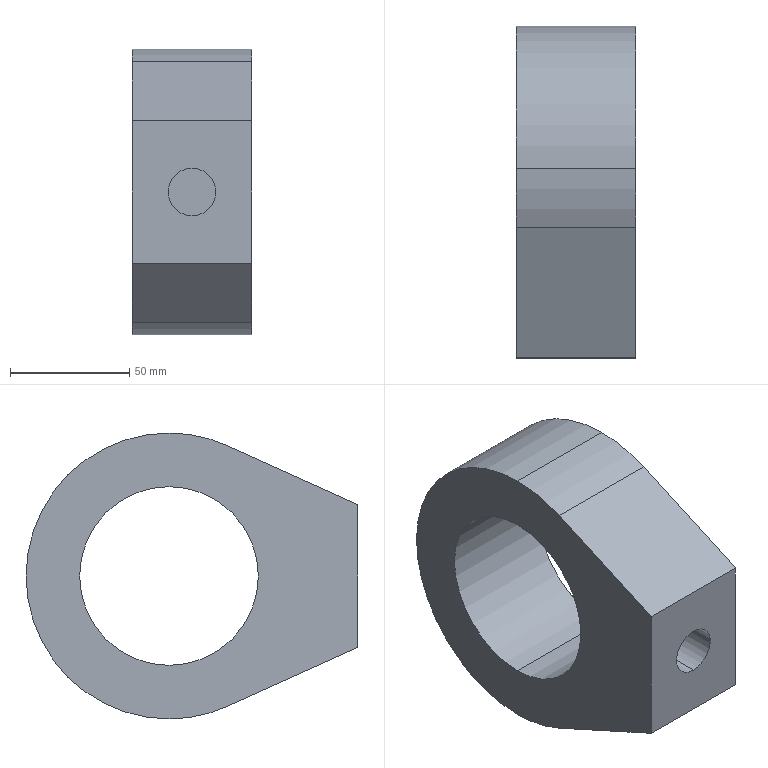Part | SolidWorks | features BaseBody 1 | 1 solid | 13 faces | box 50 x 139.314 x 120 mm | volume 424421 mm3 | cylinder 7 | plane 6 | commonest cylinder face diameters 120 x3 20 x2 75 x2
STEP:
#1=CARTESIAN_POINT('',(50.,0.,60.));
#2=VERTEX_POINT('',#1);
#3=CARTESIAN_POINT('',(50.,0.,-60.));
#4=VERTEX_POINT('',#3);
#5=CARTESIAN_POINT('',(50.,0.,0.));
#6=DIRECTION('',(-1.,0.,0.));
#7=DIRECTION('',(0.,0.,1.));
#8=AXIS2_PLACEMENT_3D('',#5,#6,#7);
#9=CIRCLE('',#8,60.);
#10=EDGE_CURVE('',#2,#4,#9,.T.);
#11=ORIENTED_EDGE('',*,*,#10,.T.);
#12=CARTESIAN_POINT('',(0.,0.,-60.));
#13=VERTEX_POINT('',#12);
#14=CARTESIAN_POINT('',(50.,0.,-60.));
#15=DIRECTION('',(-1.,0.,0.));
#16=VECTOR('',#15,1000.);
#17=LINE('',#14,#16);
#18=EDGE_CURVE('',#4,#13,#17,.T.);
#19=ORIENTED_EDGE('',*,*,#18,.T.);
#20=CARTESIAN_POINT('',(0.,0.,60.));
#21=VERTEX_POINT('',#20);
#22=CARTESIAN_POINT('',(0.,0.,0.));
#23=DIRECTION('',(1.,0.,0.));
#24=DIRECTION('',(0.,0.,1.));
#25=AXIS2_PLACEMENT_3D('',#22,#23,#24);
#26=CIRCLE('',#25,60.);
#27=EDGE_CURVE('',#13,#21,#26,.T.);
#28=ORIENTED_EDGE('',*,*,#27,.T.);
#29=CARTESIAN_POINT('',(50.,0.,60.));
#30=DIRECTION('',(-1.,0.,0.));
#31=VECTOR('',#30,1000.);
#32=LINE('',#29,#31);
#33=EDGE_CURVE('',#2,#21,#32,.T.);
#34=ORIENTED_EDGE('',*,*,#33,.F.);
#35=EDGE_LOOP('',(#11,#19,#28,#34));
#36=FACE_OUTER_BOUND('',#35,.T.);
#37=CARTESIAN_POINT('',(50.,0.,0.));
#38=DIRECTION('',(-1.,0.,0.));
#39=DIRECTION('',(0.,0.,1.));
#40=AXIS2_PLACEMENT_3D('',#37,#38,#39);
#41=CYLINDRICAL_SURFACE('',#40,60.);
#42=ADVANCED_FACE('',(#36),#41,.T.);
#43=CARTESIAN_POINT('',(50.,-24.708,54.676));
#44=VERTEX_POINT('',#43);
#45=CARTESIAN_POINT('',(50.,0.,0.));
#46=DIRECTION('',(-1.,0.,0.));
#47=DIRECTION('',(0.,0.,1.));
#48=AXIS2_PLACEMENT_3D('',#45,#46,#47);
#49=CIRCLE('',#48,60.);
#50=EDGE_CURVE('',#44,#2,#49,.T.);
#51=ORIENTED_EDGE('',*,*,#50,.T.);
#52=ORIENTED_EDGE('',*,*,#33,.T.);
#53=CARTESIAN_POINT('',(0.,-24.708,54.676));
#54=VERTEX_POINT('',#53);
#55=CARTESIAN_POINT('',(0.,0.,0.));
#56=DIRECTION('',(1.,0.,0.));
#57=DIRECTION('',(0.,0.,1.));
#58=AXIS2_PLACEMENT_3D('',#55,#56,#57);
#59=CIRCLE('',#58,60.);
#60=EDGE_CURVE('',#21,#54,#59,.T.);
#61=ORIENTED_EDGE('',*,*,#60,.T.);
#62=CARTESIAN_POINT('',(50.,-24.708,54.676));
#63=DIRECTION('',(1.,0.,0.));
#64=VECTOR('',#63,1000.);
#65=LINE('',#62,#64);
#66=EDGE_CURVE('',#54,#44,#65,.T.);
#67=ORIENTED_EDGE('',*,*,#66,.T.);
#68=EDGE_LOOP('',(#51,#52,#61,#67));
#69=FACE_OUTER_BOUND('',#68,.T.);
#70=CARTESIAN_POINT('',(50.,0.,0.));
#71=DIRECTION('',(-1.,0.,0.));
#72=DIRECTION('',(0.,0.,1.));
#73=AXIS2_PLACEMENT_3D('',#70,#71,#72);
#74=CYLINDRICAL_SURFACE('',#73,60.);
#75=ADVANCED_FACE('',(#69),#74,.T.);
#76=CARTESIAN_POINT('',(50.,0.,-37.5));
#77=VERTEX_POINT('',#76);
#78=CARTESIAN_POINT('',(50.,0.,37.5));
#79=VERTEX_POINT('',#78);
#80=CARTESIAN_POINT('',(50.,0.,0.));
#81=DIRECTION('',(-1.,0.,0.));
#82=DIRECTION('',(0.,0.,1.));
#83=AXIS2_PLACEMENT_3D('',#80,#81,#82);
#84=CIRCLE('',#83,37.5);
#85=EDGE_CURVE('',#77,#79,#84,.T.);
#86=ORIENTED_EDGE('',*,*,#85,.F.);
#87=CARTESIAN_POINT('',(0.,0.,-37.5));
#88=VERTEX_POINT('',#87);
#89=CARTESIAN_POINT('',(50.,0.,-37.5));
#90=DIRECTION('',(-1.,0.,0.));
#91=VECTOR('',#90,1000.);
#92=LINE('',#89,#91);
#93=EDGE_CURVE('',#77,#88,#92,.T.);
#94=ORIENTED_EDGE('',*,*,#93,.T.);
#95=CARTESIAN_POINT('',(0.,0.,37.5));
#96=VERTEX_POINT('',#95);
#97=CARTESIAN_POINT('',(0.,0.,0.));
#98=DIRECTION('',(-1.,0.,0.));
#99=DIRECTION('',(0.,0.,1.));
#100=AXIS2_PLACEMENT_3D('',#97,#98,#99);
#101=CIRCLE('',#100,37.5);
#102=EDGE_CURVE('',#88,#96,#101,.T.);
#103=ORIENTED_EDGE('',*,*,#102,.T.);
#104=CARTESIAN_POINT('',(50.,0.,37.5));
#105=DIRECTION('',(-1.,0.,0.));
#106=VECTOR('',#105,1000.);
#107=LINE('',#104,#106);
#108=EDGE_CURVE('',#79,#96,#107,.T.);
#109=ORIENTED_EDGE('',*,*,#108,.F.);
#110=EDGE_LOOP('',(#86,#94,#103,#109));
#111=FACE_OUTER_BOUND('',#110,.T.);
#112=CARTESIAN_POINT('',(50.,0.,0.));
#113=DIRECTION('',(-1.,0.,0.));
#114=DIRECTION('',(0.,0.,1.));
#115=AXIS2_PLACEMENT_3D('',#112,#113,#114);
#116=CYLINDRICAL_SURFACE('',#115,37.5);
#117=ADVANCED_FACE('',(#111),#116,.F.);
#118=CARTESIAN_POINT('',(25.,-39.314,10.));
#119=VERTEX_POINT('',#118);
#120=CARTESIAN_POINT('',(25.,-39.314,-10.));
#121=VERTEX_POINT('',#120);
#122=CARTESIAN_POINT('',(25.,-39.314,0.));
#123=DIRECTION('',(0.,-1.,0.));
#124=DIRECTION('',(0.,0.,-1.));
#125=AXIS2_PLACEMENT_3D('',#122,#123,#124);
#126=CIRCLE('',#125,10.);
#127=EDGE_CURVE('',#119,#121,#126,.T.);
#128=ORIENTED_EDGE('',*,*,#127,.F.);
#129=CARTESIAN_POINT('',(25.,-79.314,10.));
#130=VERTEX_POINT('',#129);
#131=CARTESIAN_POINT('',(25.,-39.314,10.));
#132=DIRECTION('',(0.,-1.,0.));
#133=VECTOR('',#132,1000.);
#134=LINE('',#131,#133);
#135=EDGE_CURVE('',#119,#130,#134,.T.);
#136=ORIENTED_EDGE('',*,*,#135,.T.);
#137=CARTESIAN_POINT('',(25.,-79.314,-10.));
#138=VERTEX_POINT('',#137);
#139=CARTESIAN_POINT('',(25.,-79.314,0.));
#140=DIRECTION('',(0.,-1.,0.));
#141=DIRECTION('',(0.,0.,-1.));
#142=AXIS2_PLACEMENT_3D('',#139,#140,#141);
#143=CIRCLE('',#142,10.);
#144=EDGE_CURVE('',#130,#138,#143,.T.);
#145=ORIENTED_EDGE('',*,*,#144,.T.);
#146=CARTESIAN_POINT('',(25.,-39.314,-10.));
#147=DIRECTION('',(0.,-1.,0.));
#148=VECTOR('',#147,1000.);
#149=LINE('',#146,#148);
#150=EDGE_CURVE('',#121,#138,#149,.T.);
#151=ORIENTED_EDGE('',*,*,#150,.F.);
#152=EDGE_LOOP('',(#128,#136,#145,#151));
#153=FACE_OUTER_BOUND('',#152,.T.);
#154=CARTESIAN_POINT('',(25.,-39.314,0.));
#155=DIRECTION('',(0.,-1.,0.));
#156=DIRECTION('',(0.,0.,-1.));
#157=AXIS2_PLACEMENT_3D('',#154,#155,#156);
#158=CYLINDRICAL_SURFACE('',#157,10.);
#159=ADVANCED_FACE('',(#153),#158,.F.);
#160=ORIENTED_EDGE('',*,*,#18,.F.);
#161=CARTESIAN_POINT('',(50.,-24.708,-54.676));
#162=VERTEX_POINT('',#161);
#163=CARTESIAN_POINT('',(50.,0.,0.));
#164=DIRECTION('',(-1.,0.,0.));
#165=DIRECTION('',(0.,0.,1.));
#166=AXIS2_PLACEMENT_3D('',#163,#164,#165);
#167=CIRCLE('',#166,60.);
#168=EDGE_CURVE('',#4,#162,#167,.T.);
#169=ORIENTED_EDGE('',*,*,#168,.T.);
#170=CARTESIAN_POINT('',(0.,-24.708,-54.676));
#171=VERTEX_POINT('',#170);
#172=CARTESIAN_POINT('',(50.,-24.708,-54.676));
#173=DIRECTION('',(-1.,0.,0.));
#174=VECTOR('',#173,1000.);
#175=LINE('',#172,#174);
#176=EDGE_CURVE('',#162,#171,#175,.T.);
#177=ORIENTED_EDGE('',*,*,#176,.T.);
#178=CARTESIAN_POINT('',(0.,0.,0.));
#179=DIRECTION('',(1.,0.,0.));
#180=DIRECTION('',(0.,0.,1.));
#181=AXIS2_PLACEMENT_3D('',#178,#179,#180);
#182=CIRCLE('',#181,60.);
#183=EDGE_CURVE('',#171,#13,#182,.T.);
#184=ORIENTED_EDGE('',*,*,#183,.T.);
#185=EDGE_LOOP('',(#160,#169,#177,#184));
#186=FACE_OUTER_BOUND('',#185,.T.);
#187=CARTESIAN_POINT('',(50.,0.,0.));
#188=DIRECTION('',(-1.,0.,0.));
#189=DIRECTION('',(0.,0.,1.));
#190=AXIS2_PLACEMENT_3D('',#187,#188,#189);
#191=CYLINDRICAL_SURFACE('',#190,60.);
#192=ADVANCED_FACE('',(#186),#191,.T.);
#193=CARTESIAN_POINT('',(0.,0.,0.));
#194=DIRECTION('',(-1.,0.,0.));
#195=DIRECTION('',(0.,0.,1.));
#196=AXIS2_PLACEMENT_3D('',#193,#194,#195);
#197=CIRCLE('',#196,37.5);
#198=EDGE_CURVE('',#96,#88,#197,.T.);
#199=ORIENTED_EDGE('',*,*,#198,.F.);
#200=ORIENTED_EDGE('',*,*,#102,.F.);
#201=EDGE_LOOP('',(#199,#200));
#202=FACE_BOUND('',#201,.T.);
#203=CARTESIAN_POINT('',(0.,-79.314,30.));
#204=VERTEX_POINT('',#203);
#205=CARTESIAN_POINT('',(0.,-24.708,54.676));
#206=DIRECTION('',(0.,-0.9113,-0.4118));
#207=VECTOR('',#206,1000.);
#208=LINE('',#205,#207);
#209=EDGE_CURVE('',#54,#204,#208,.T.);
#210=ORIENTED_EDGE('',*,*,#209,.F.);
#211=ORIENTED_EDGE('',*,*,#60,.F.);
#212=ORIENTED_EDGE('',*,*,#27,.F.);
#213=ORIENTED_EDGE('',*,*,#183,.F.);
#214=CARTESIAN_POINT('',(0.,-79.314,-30.));
#215=VERTEX_POINT('',#214);
#216=CARTESIAN_POINT('',(0.,-79.314,-30.));
#217=DIRECTION('',(0.,0.9113,-0.4118));
#218=VECTOR('',#217,1000.);
#219=LINE('',#216,#218);
#220=EDGE_CURVE('',#215,#171,#219,.T.);
#221=ORIENTED_EDGE('',*,*,#220,.F.);
#222=CARTESIAN_POINT('',(0.,-79.314,0.));
#223=DIRECTION('',(0.,0.,-1.));
#224=VECTOR('',#223,1000.);
#225=LINE('',#222,#224);
#226=EDGE_CURVE('',#204,#215,#225,.T.);
#227=ORIENTED_EDGE('',*,*,#226,.F.);
#228=EDGE_LOOP('',(#210,#211,#212,#213,#221,#227));
#229=FACE_OUTER_BOUND('',#228,.T.);
#230=CARTESIAN_POINT('',(0.,0.,0.));
#231=DIRECTION('',(1.,0.,0.));
#232=DIRECTION('',(0.,0.,-1.));
#233=AXIS2_PLACEMENT_3D('',#230,#231,#232);
#234=PLANE('',#233);
#235=ADVANCED_FACE('',(#202,#229),#234,.F.);
#236=CARTESIAN_POINT('',(50.,0.,0.));
#237=DIRECTION('',(-1.,0.,0.));
#238=DIRECTION('',(0.,0.,1.));
#239=AXIS2_PLACEMENT_3D('',#236,#237,#238);
#240=CIRCLE('',#239,37.5);
#241=EDGE_CURVE('',#79,#77,#240,.T.);
#242=ORIENTED_EDGE('',*,*,#241,.T.);
#243=ORIENTED_EDGE('',*,*,#85,.T.);
#244=EDGE_LOOP('',(#242,#243));
#245=FACE_BOUND('',#244,.T.);
#246=ORIENTED_EDGE('',*,*,#50,.F.);
#247=CARTESIAN_POINT('',(50.,-79.314,30.));
#248=VERTEX_POINT('',#247);
#249=CARTESIAN_POINT('',(50.,-24.708,54.676));
#250=DIRECTION('',(0.,-0.9113,-0.4118));
#251=VECTOR('',#250,1000.);
#252=LINE('',#249,#251);
#253=EDGE_CURVE('',#44,#248,#252,.T.);
#254=ORIENTED_EDGE('',*,*,#253,.T.);
#255=CARTESIAN_POINT('',(50.,-79.314,-30.));
#256=VERTEX_POINT('',#255);
#257=CARTESIAN_POINT('',(50.,-79.314,0.));
#258=DIRECTION('',(0.,0.,-1.));
#259=VECTOR('',#258,1000.);
#260=LINE('',#257,#259);
#261=EDGE_CURVE('',#248,#256,#260,.T.);
#262=ORIENTED_EDGE('',*,*,#261,.T.);
#263=CARTESIAN_POINT('',(50.,-79.314,-30.));
#264=DIRECTION('',(0.,0.9113,-0.4118));
#265=VECTOR('',#264,1000.);
#266=LINE('',#263,#265);
#267=EDGE_CURVE('',#256,#162,#266,.T.);
#268=ORIENTED_EDGE('',*,*,#267,.T.);
#269=ORIENTED_EDGE('',*,*,#168,.F.);
#270=ORIENTED_EDGE('',*,*,#10,.F.);
#271=EDGE_LOOP('',(#246,#254,#262,#268,#269,#270));
#272=FACE_OUTER_BOUND('',#271,.T.);
#273=CARTESIAN_POINT('',(50.,0.,0.));
#274=DIRECTION('',(1.,0.,0.));
#275=DIRECTION('',(0.,0.,-1.));
#276=AXIS2_PLACEMENT_3D('',#273,#274,#275);
#277=PLANE('',#276);
#278=ADVANCED_FACE('',(#245,#272),#277,.T.);
#279=CARTESIAN_POINT('',(50.,-79.314,30.));
#280=DIRECTION('',(-1.,0.,0.));
#281=VECTOR('',#280,1000.);
#282=LINE('',#279,#281);
#283=EDGE_CURVE('',#248,#204,#282,.T.);
#284=ORIENTED_EDGE('',*,*,#283,.F.);
#285=ORIENTED_EDGE('',*,*,#253,.F.);
#286=ORIENTED_EDGE('',*,*,#66,.F.);
#287=ORIENTED_EDGE('',*,*,#209,.T.);
#288=EDGE_LOOP('',(#284,#285,#286,#287));
#289=FACE_OUTER_BOUND('',#288,.T.);
#290=CARTESIAN_POINT('',(50.,-24.708,54.676));
#291=DIRECTION('',(0.,0.4118,-0.9113));
#292=DIRECTION('',(0.,0.9113,0.4118));
#293=AXIS2_PLACEMENT_3D('',#290,#291,#292);
#294=PLANE('',#293);
#295=ADVANCED_FACE('',(#289),#294,.F.);
#296=ORIENTED_EDGE('',*,*,#93,.F.);
#297=ORIENTED_EDGE('',*,*,#241,.F.);
#298=ORIENTED_EDGE('',*,*,#108,.T.);
#299=ORIENTED_EDGE('',*,*,#198,.T.);
#300=EDGE_LOOP('',(#296,#297,#298,#299));
#301=FACE_OUTER_BOUND('',#300,.T.);
#302=CARTESIAN_POINT('',(50.,0.,0.));
#303=DIRECTION('',(-1.,0.,0.));
#304=DIRECTION('',(0.,0.,1.));
#305=AXIS2_PLACEMENT_3D('',#302,#303,#304);
#306=CYLINDRICAL_SURFACE('',#305,37.5);
#307=ADVANCED_FACE('',(#301),#306,.F.);
#308=ORIENTED_EDGE('',*,*,#176,.F.);
#309=ORIENTED_EDGE('',*,*,#267,.F.);
#310=CARTESIAN_POINT('',(50.,-79.314,-30.));
#311=DIRECTION('',(1.,0.,0.));
#312=VECTOR('',#311,1000.);
#313=LINE('',#310,#312);
#314=EDGE_CURVE('',#215,#256,#313,.T.);
#315=ORIENTED_EDGE('',*,*,#314,.F.);
#316=ORIENTED_EDGE('',*,*,#220,.T.);
#317=EDGE_LOOP('',(#308,#309,#315,#316));
#318=FACE_OUTER_BOUND('',#317,.T.);
#319=CARTESIAN_POINT('',(50.,-79.314,-30.));
#320=DIRECTION('',(0.,0.4118,0.9113));
#321=DIRECTION('',(0.,-0.9113,0.4118));
#322=AXIS2_PLACEMENT_3D('',#319,#320,#321);
#323=PLANE('',#322);
#324=ADVANCED_FACE('',(#318),#323,.F.);
#325=ORIENTED_EDGE('',*,*,#314,.T.);
#326=ORIENTED_EDGE('',*,*,#261,.F.);
#327=ORIENTED_EDGE('',*,*,#283,.T.);
#328=ORIENTED_EDGE('',*,*,#226,.T.);
#329=EDGE_LOOP('',(#325,#326,#327,#328));
#330=FACE_OUTER_BOUND('',#329,.T.);
#331=CARTESIAN_POINT('',(25.,-79.314,0.));
#332=DIRECTION('',(0.,-1.,0.));
#333=DIRECTION('',(0.,0.,-1.));
#334=AXIS2_PLACEMENT_3D('',#331,#332,#333);
#335=CIRCLE('',#334,10.);
#336=EDGE_CURVE('',#138,#130,#335,.T.);
#337=ORIENTED_EDGE('',*,*,#336,.F.);
#338=ORIENTED_EDGE('',*,*,#144,.F.);
#339=EDGE_LOOP('',(#337,#338));
#340=FACE_BOUND('',#339,.T.);
#341=CARTESIAN_POINT('',(50.,-79.314,30.));
#342=DIRECTION('',(0.,1.,0.));
#343=DIRECTION('',(0.,0.,1.));
#344=AXIS2_PLACEMENT_3D('',#341,#342,#343);
#345=PLANE('',#344);
#346=ADVANCED_FACE('',(#330,#340),#345,.F.);
#347=ORIENTED_EDGE('',*,*,#135,.F.);
#348=CARTESIAN_POINT('',(25.,-39.314,0.));
#349=DIRECTION('',(0.,-1.,0.));
#350=DIRECTION('',(0.,0.,-1.));
#351=AXIS2_PLACEMENT_3D('',#348,#349,#350);
#352=CIRCLE('',#351,10.);
#353=EDGE_CURVE('',#121,#119,#352,.T.);
#354=ORIENTED_EDGE('',*,*,#353,.F.);
#355=ORIENTED_EDGE('',*,*,#150,.T.);
#356=ORIENTED_EDGE('',*,*,#336,.T.);
#357=EDGE_LOOP('',(#347,#354,#355,#356));
#358=FACE_OUTER_BOUND('',#357,.T.);
#359=CARTESIAN_POINT('',(25.,-39.314,0.));
#360=DIRECTION('',(0.,-1.,0.));
#361=DIRECTION('',(0.,0.,-1.));
#362=AXIS2_PLACEMENT_3D('',#359,#360,#361);
#363=CYLINDRICAL_SURFACE('',#362,10.);
#364=ADVANCED_FACE('',(#358),#363,.F.);
#365=ORIENTED_EDGE('',*,*,#353,.T.);
#366=ORIENTED_EDGE('',*,*,#127,.T.);
#367=EDGE_LOOP('',(#365,#366));
#368=FACE_OUTER_BOUND('',#367,.T.);
#369=CARTESIAN_POINT('',(25.,-39.314,0.));
#370=DIRECTION('',(0.,-1.,0.));
#371=DIRECTION('',(0.,0.,-1.));
#372=AXIS2_PLACEMENT_3D('',#369,#370,#371);
#373=PLANE('',#372);
#374=ADVANCED_FACE('',(#368),#373,.T.);
#375=CLOSED_SHELL('',(#42,#75,#117,#159,#192,#235,#278,#295,#307,#324,#346,#364,#374));
#376=MANIFOLD_SOLID_BREP('',#375);
#377=CARTESIAN_POINT('',(0.,0.,0.));
#378=DIRECTION('',(0.,0.,1.));
#379=DIRECTION('',(1.,0.,0.));
#380=AXIS2_PLACEMENT_3D('',#377,#378,#379);
#381=(LENGTH_UNIT()NAMED_UNIT(*)SI_UNIT(.MILLI.,.METRE.));
#382=UNCERTAINTY_MEASURE_WITH_UNIT(LENGTH_MEASURE(0.00001),#381,'','');
#383=(NAMED_UNIT(*)PLANE_ANGLE_UNIT()SI_UNIT($,.RADIAN.));
#384=(NAMED_UNIT(*)SI_UNIT($,.STERADIAN.)SOLID_ANGLE_UNIT());
#385=(GEOMETRIC_REPRESENTATION_CONTEXT(3)GLOBAL_UNCERTAINTY_ASSIGNED_CONTEXT((#382))GLOBAL_UNIT_ASSIGNED_CONTEXT((#381,#383,#384))REPRESENTATION_CONTEXT('',''));
#386=ADVANCED_BREP_SHAPE_REPRESENTATION('',(#376,#380),#385);